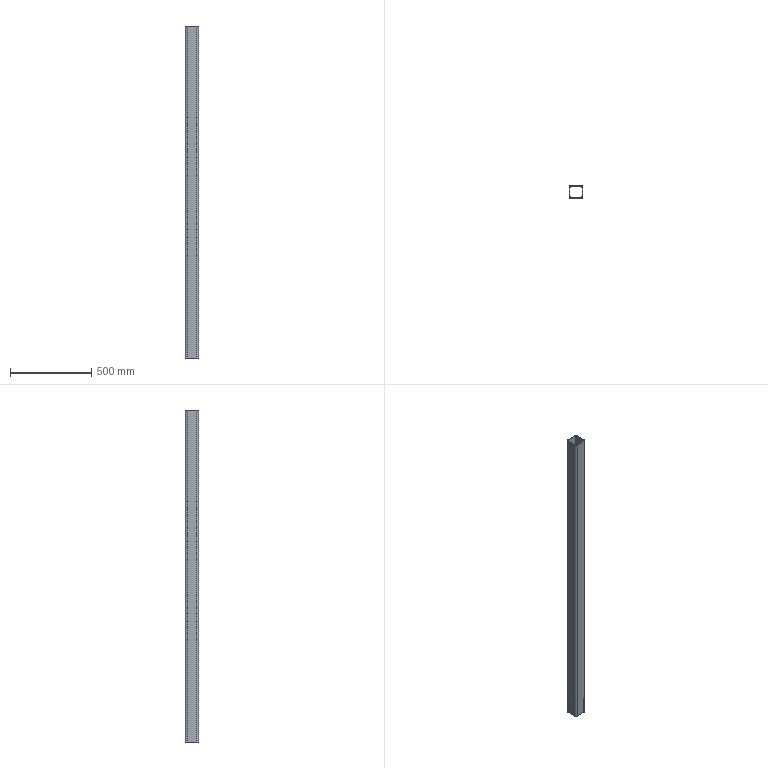Part | STEP file | 1 solid | 18 faces | box 80 x 80 x 2040 mm | volume 1795651 mm3 | plane 10 | cylinder 8 | commonest cylinder face diameters 14 x4 20 x4
STEP:
#1=CARTESIAN_POINT('',(0.,0.,0.));
#2=DIRECTION('',(0.,0.,1.));
#3=DIRECTION('',(1.,0.,0.));
#4=AXIS2_PLACEMENT_3D('',#1,#2,#3);
#5=CARTESIAN_POINT('',(-30.,40.,1020.));
#6=VERTEX_POINT('',#5);
#7=CARTESIAN_POINT('',(-40.,30.,1020.));
#8=VERTEX_POINT('',#7);
#9=CARTESIAN_POINT('',(-30.,30.,1020.));
#10=DIRECTION('',(0.,0.,1.));
#11=DIRECTION('',(1.,0.,0.));
#12=AXIS2_PLACEMENT_3D('',#9,#10,#11);
#13=CIRCLE('',#12,10.);
#14=CARTESIAN_POINT('',(-30.,30.,1020.));
#15=DIRECTION('',(0.,0.,1.));
#16=DIRECTION('',(1.,0.,0.));
#17=AXIS2_PLACEMENT_3D('',#14,#15,#16);
#18=PLANE('',#17);
#19=CARTESIAN_POINT('',(0.,0.));
#20=DIRECTION('',(1.,0.));
#21=AXIS2_PLACEMENT_2D('',#19,#20);
#22=CIRCLE('',#21,10.);
#23=(GEOMETRIC_REPRESENTATION_CONTEXT(2)PARAMETRIC_REPRESENTATION_CONTEXT()REPRESENTATION_CONTEXT('',''));
#24=DEFINITIONAL_REPRESENTATION('',(#22),#23);
#25=PCURVE('',#18,#24);
#26=CARTESIAN_POINT('',(-30.,30.,1020.));
#27=DIRECTION('',(0.,0.,-1.));
#28=DIRECTION('',(-1.,0.,0.));
#29=AXIS2_PLACEMENT_3D('',#26,#27,#28);
#30=CYLINDRICAL_SURFACE('',#29,10.);
#31=CARTESIAN_POINT('',(3.142,0.));
#32=DIRECTION('',(-1.,0.));
#33=VECTOR('',#32,1.);
#34=LINE('',#31,#33);
#35=(GEOMETRIC_REPRESENTATION_CONTEXT(2)PARAMETRIC_REPRESENTATION_CONTEXT()REPRESENTATION_CONTEXT('',''));
#36=DEFINITIONAL_REPRESENTATION('',(#34),#35);
#37=PCURVE('',#30,#36);
#38=SURFACE_CURVE('',#13,(#25,#37),.PCURVE_S1.);
#39=EDGE_CURVE('',#6,#8,#38,.T.);
#40=ORIENTED_EDGE('',*,*,#39,.T.);
#41=CARTESIAN_POINT('',(-40.,-30.,1020.));
#42=VERTEX_POINT('',#41);
#43=CARTESIAN_POINT('',(-40.,30.,1020.));
#44=DIRECTION('',(0.,-1.,0.));
#45=VECTOR('',#44,1.);
#46=LINE('',#43,#45);
#47=CARTESIAN_POINT('',(-10.,0.));
#48=DIRECTION('',(0.,-1.));
#49=VECTOR('',#48,1.);
#50=LINE('',#47,#49);
#51=(GEOMETRIC_REPRESENTATION_CONTEXT(2)PARAMETRIC_REPRESENTATION_CONTEXT()REPRESENTATION_CONTEXT('',''));
#52=DEFINITIONAL_REPRESENTATION('',(#50),#51);
#53=PCURVE('',#18,#52);
#54=CARTESIAN_POINT('',(-40.,30.,1020.));
#55=DIRECTION('',(1.,0.,0.));
#56=DIRECTION('',(0.,1.,0.));
#57=AXIS2_PLACEMENT_3D('',#54,#55,#56);
#58=PLANE('',#57);
#59=CARTESIAN_POINT('',(0.,0.));
#60=DIRECTION('',(-1.,0.));
#61=VECTOR('',#60,1.);
#62=LINE('',#59,#61);
#63=(GEOMETRIC_REPRESENTATION_CONTEXT(2)PARAMETRIC_REPRESENTATION_CONTEXT()REPRESENTATION_CONTEXT('',''));
#64=DEFINITIONAL_REPRESENTATION('',(#62),#63);
#65=PCURVE('',#58,#64);
#66=SURFACE_CURVE('',#46,(#53,#65),.PCURVE_S1.);
#67=EDGE_CURVE('',#8,#42,#66,.T.);
#68=ORIENTED_EDGE('',*,*,#67,.T.);
#69=CARTESIAN_POINT('',(-30.,-40.,1020.));
#70=VERTEX_POINT('',#69);
#71=CARTESIAN_POINT('',(-30.,-30.,1020.));
#72=DIRECTION('',(0.,0.,1.));
#73=DIRECTION('',(-1.,0.,0.));
#74=AXIS2_PLACEMENT_3D('',#71,#72,#73);
#75=CIRCLE('',#74,10.);
#76=CARTESIAN_POINT('',(0.,-60.));
#77=DIRECTION('',(-1.,0.));
#78=AXIS2_PLACEMENT_2D('',#76,#77);
#79=CIRCLE('',#78,10.);
#80=(GEOMETRIC_REPRESENTATION_CONTEXT(2)PARAMETRIC_REPRESENTATION_CONTEXT()REPRESENTATION_CONTEXT('',''));
#81=DEFINITIONAL_REPRESENTATION('',(#79),#80);
#82=PCURVE('',#18,#81);
#83=CARTESIAN_POINT('',(-30.,-30.,1020.));
#84=DIRECTION('',(0.,0.,-1.));
#85=DIRECTION('',(-1.,0.,0.));
#86=AXIS2_PLACEMENT_3D('',#83,#84,#85);
#87=CYLINDRICAL_SURFACE('',#86,10.);
#88=CARTESIAN_POINT('',(6.283,0.));
#89=DIRECTION('',(-1.,0.));
#90=VECTOR('',#89,1.);
#91=LINE('',#88,#90);
#92=(GEOMETRIC_REPRESENTATION_CONTEXT(2)PARAMETRIC_REPRESENTATION_CONTEXT()REPRESENTATION_CONTEXT('',''));
#93=DEFINITIONAL_REPRESENTATION('',(#91),#92);
#94=PCURVE('',#87,#93);
#95=SURFACE_CURVE('',#75,(#82,#94),.PCURVE_S1.);
#96=EDGE_CURVE('',#42,#70,#95,.T.);
#97=ORIENTED_EDGE('',*,*,#96,.T.);
#98=CARTESIAN_POINT('',(30.,-40.,1020.));
#99=VERTEX_POINT('',#98);
#100=CARTESIAN_POINT('',(30.,-40.,1020.));
#101=DIRECTION('',(1.,0.,0.));
#102=VECTOR('',#101,1.);
#103=LINE('',#100,#102);
#104=CARTESIAN_POINT('',(60.,-70.));
#105=DIRECTION('',(1.,0.));
#106=VECTOR('',#105,1.);
#107=LINE('',#104,#106);
#108=(GEOMETRIC_REPRESENTATION_CONTEXT(2)PARAMETRIC_REPRESENTATION_CONTEXT()REPRESENTATION_CONTEXT('',''));
#109=DEFINITIONAL_REPRESENTATION('',(#107),#108);
#110=PCURVE('',#18,#109);
#111=CARTESIAN_POINT('',(30.,-40.,1020.));
#112=DIRECTION('',(0.,1.,0.));
#113=DIRECTION('',(-1.,0.,0.));
#114=AXIS2_PLACEMENT_3D('',#111,#112,#113);
#115=PLANE('',#114);
#116=CARTESIAN_POINT('',(0.,0.));
#117=DIRECTION('',(-1.,0.));
#118=VECTOR('',#117,1.);
#119=LINE('',#116,#118);
#120=(GEOMETRIC_REPRESENTATION_CONTEXT(2)PARAMETRIC_REPRESENTATION_CONTEXT()REPRESENTATION_CONTEXT('',''));
#121=DEFINITIONAL_REPRESENTATION('',(#119),#120);
#122=PCURVE('',#115,#121);
#123=SURFACE_CURVE('',#103,(#110,#122),.PCURVE_S1.);
#124=EDGE_CURVE('',#70,#99,#123,.T.);
#125=ORIENTED_EDGE('',*,*,#124,.T.);
#126=CARTESIAN_POINT('',(40.,-30.,1020.));
#127=VERTEX_POINT('',#126);
#128=CARTESIAN_POINT('',(30.,-30.,1020.));
#129=DIRECTION('',(0.,0.,1.));
#130=DIRECTION('',(-1.,0.,0.));
#131=AXIS2_PLACEMENT_3D('',#128,#129,#130);
#132=CIRCLE('',#131,10.);
#133=CARTESIAN_POINT('',(60.,-60.));
#134=DIRECTION('',(-1.,0.));
#135=AXIS2_PLACEMENT_2D('',#133,#134);
#136=CIRCLE('',#135,10.);
#137=(GEOMETRIC_REPRESENTATION_CONTEXT(2)PARAMETRIC_REPRESENTATION_CONTEXT()REPRESENTATION_CONTEXT('',''));
#138=DEFINITIONAL_REPRESENTATION('',(#136),#137);
#139=PCURVE('',#18,#138);
#140=CARTESIAN_POINT('',(30.,-30.,1020.));
#141=DIRECTION('',(0.,0.,-1.));
#142=DIRECTION('',(-1.,0.,0.));
#143=AXIS2_PLACEMENT_3D('',#140,#141,#142);
#144=CYLINDRICAL_SURFACE('',#143,10.);
#145=CARTESIAN_POINT('',(6.283,0.));
#146=DIRECTION('',(-1.,0.));
#147=VECTOR('',#146,1.);
#148=LINE('',#145,#147);
#149=(GEOMETRIC_REPRESENTATION_CONTEXT(2)PARAMETRIC_REPRESENTATION_CONTEXT()REPRESENTATION_CONTEXT('',''));
#150=DEFINITIONAL_REPRESENTATION('',(#148),#149);
#151=PCURVE('',#144,#150);
#152=SURFACE_CURVE('',#132,(#139,#151),.PCURVE_S1.);
#153=EDGE_CURVE('',#99,#127,#152,.T.);
#154=ORIENTED_EDGE('',*,*,#153,.T.);
#155=CARTESIAN_POINT('',(40.,30.,1020.));
#156=VERTEX_POINT('',#155);
#157=CARTESIAN_POINT('',(40.,30.,1020.));
#158=DIRECTION('',(0.,1.,0.));
#159=VECTOR('',#158,1.);
#160=LINE('',#157,#159);
#161=CARTESIAN_POINT('',(70.,0.));
#162=DIRECTION('',(0.,1.));
#163=VECTOR('',#162,1.);
#164=LINE('',#161,#163);
#165=(GEOMETRIC_REPRESENTATION_CONTEXT(2)PARAMETRIC_REPRESENTATION_CONTEXT()REPRESENTATION_CONTEXT('',''));
#166=DEFINITIONAL_REPRESENTATION('',(#164),#165);
#167=PCURVE('',#18,#166);
#168=CARTESIAN_POINT('',(40.,30.,1020.));
#169=DIRECTION('',(-1.,0.,0.));
#170=DIRECTION('',(0.,-1.,0.));
#171=AXIS2_PLACEMENT_3D('',#168,#169,#170);
#172=PLANE('',#171);
#173=CARTESIAN_POINT('',(0.,0.));
#174=DIRECTION('',(-1.,0.));
#175=VECTOR('',#174,1.);
#176=LINE('',#173,#175);
#177=(GEOMETRIC_REPRESENTATION_CONTEXT(2)PARAMETRIC_REPRESENTATION_CONTEXT()REPRESENTATION_CONTEXT('',''));
#178=DEFINITIONAL_REPRESENTATION('',(#176),#177);
#179=PCURVE('',#172,#178);
#180=SURFACE_CURVE('',#160,(#167,#179),.PCURVE_S1.);
#181=EDGE_CURVE('',#127,#156,#180,.T.);
#182=ORIENTED_EDGE('',*,*,#181,.T.);
#183=CARTESIAN_POINT('',(30.,40.,1020.));
#184=VERTEX_POINT('',#183);
#185=CARTESIAN_POINT('',(30.,30.,1020.));
#186=DIRECTION('',(0.,0.,1.));
#187=DIRECTION('',(-1.,0.,0.));
#188=AXIS2_PLACEMENT_3D('',#185,#186,#187);
#189=CIRCLE('',#188,10.);
#190=CARTESIAN_POINT('',(60.,0.));
#191=DIRECTION('',(-1.,0.));
#192=AXIS2_PLACEMENT_2D('',#190,#191);
#193=CIRCLE('',#192,10.);
#194=(GEOMETRIC_REPRESENTATION_CONTEXT(2)PARAMETRIC_REPRESENTATION_CONTEXT()REPRESENTATION_CONTEXT('',''));
#195=DEFINITIONAL_REPRESENTATION('',(#193),#194);
#196=PCURVE('',#18,#195);
#197=CARTESIAN_POINT('',(30.,30.,1020.));
#198=DIRECTION('',(0.,0.,-1.));
#199=DIRECTION('',(-1.,0.,0.));
#200=AXIS2_PLACEMENT_3D('',#197,#198,#199);
#201=CYLINDRICAL_SURFACE('',#200,10.);
#202=CARTESIAN_POINT('',(6.283,0.));
#203=DIRECTION('',(-1.,0.));
#204=VECTOR('',#203,1.);
#205=LINE('',#202,#204);
#206=(GEOMETRIC_REPRESENTATION_CONTEXT(2)PARAMETRIC_REPRESENTATION_CONTEXT()REPRESENTATION_CONTEXT('',''));
#207=DEFINITIONAL_REPRESENTATION('',(#205),#206);
#208=PCURVE('',#201,#207);
#209=SURFACE_CURVE('',#189,(#196,#208),.PCURVE_S1.);
#210=EDGE_CURVE('',#156,#184,#209,.T.);
#211=ORIENTED_EDGE('',*,*,#210,.T.);
#212=CARTESIAN_POINT('',(30.,40.,1020.));
#213=DIRECTION('',(-1.,0.,0.));
#214=VECTOR('',#213,1.);
#215=LINE('',#212,#214);
#216=CARTESIAN_POINT('',(60.,10.));
#217=DIRECTION('',(-1.,0.));
#218=VECTOR('',#217,1.);
#219=LINE('',#216,#218);
#220=(GEOMETRIC_REPRESENTATION_CONTEXT(2)PARAMETRIC_REPRESENTATION_CONTEXT()REPRESENTATION_CONTEXT('',''));
#221=DEFINITIONAL_REPRESENTATION('',(#219),#220);
#222=PCURVE('',#18,#221);
#223=CARTESIAN_POINT('',(30.,40.,1020.));
#224=DIRECTION('',(0.,-1.,0.));
#225=DIRECTION('',(1.,0.,0.));
#226=AXIS2_PLACEMENT_3D('',#223,#224,#225);
#227=PLANE('',#226);
#228=CARTESIAN_POINT('',(0.,0.));
#229=DIRECTION('',(-1.,0.));
#230=VECTOR('',#229,1.);
#231=LINE('',#228,#230);
#232=(GEOMETRIC_REPRESENTATION_CONTEXT(2)PARAMETRIC_REPRESENTATION_CONTEXT()REPRESENTATION_CONTEXT('',''));
#233=DEFINITIONAL_REPRESENTATION('',(#231),#232);
#234=PCURVE('',#227,#233);
#235=SURFACE_CURVE('',#215,(#222,#234),.PCURVE_S1.);
#236=EDGE_CURVE('',#184,#6,#235,.T.);
#237=ORIENTED_EDGE('',*,*,#236,.T.);
#238=EDGE_LOOP('',(#40,#68,#97,#125,#154,#182,#211,#237));
#239=FACE_BOUND('',#238,.T.);
#240=CARTESIAN_POINT('',(30.,37.,1020.));
#241=VERTEX_POINT('',#240);
#242=CARTESIAN_POINT('',(-30.,37.,1020.));
#243=VERTEX_POINT('',#242);
#244=CARTESIAN_POINT('',(30.,37.,1020.));
#245=DIRECTION('',(-1.,0.,0.));
#246=VECTOR('',#245,1.);
#247=LINE('',#244,#246);
#248=CARTESIAN_POINT('',(60.,7.));
#249=DIRECTION('',(-1.,0.));
#250=VECTOR('',#249,1.);
#251=LINE('',#248,#250);
#252=(GEOMETRIC_REPRESENTATION_CONTEXT(2)PARAMETRIC_REPRESENTATION_CONTEXT()REPRESENTATION_CONTEXT('',''));
#253=DEFINITIONAL_REPRESENTATION('',(#251),#252);
#254=PCURVE('',#18,#253);
#255=CARTESIAN_POINT('',(30.,37.,1020.));
#256=DIRECTION('',(0.,-1.,0.));
#257=DIRECTION('',(0.,0.,-1.));
#258=AXIS2_PLACEMENT_3D('',#255,#256,#257);
#259=PLANE('',#258);
#260=CARTESIAN_POINT('',(0.,0.));
#261=DIRECTION('',(0.,-1.));
#262=VECTOR('',#261,1.);
#263=LINE('',#260,#262);
#264=(GEOMETRIC_REPRESENTATION_CONTEXT(2)PARAMETRIC_REPRESENTATION_CONTEXT()REPRESENTATION_CONTEXT('',''));
#265=DEFINITIONAL_REPRESENTATION('',(#263),#264);
#266=PCURVE('',#259,#265);
#267=SURFACE_CURVE('',#247,(#254,#266),.PCURVE_S1.);
#268=EDGE_CURVE('',#241,#243,#267,.T.);
#269=ORIENTED_EDGE('',*,*,#268,.F.);
#270=CARTESIAN_POINT('',(37.,30.,1020.));
#271=VERTEX_POINT('',#270);
#272=CARTESIAN_POINT('',(30.,30.,1020.));
#273=DIRECTION('',(0.,0.,1.));
#274=DIRECTION('',(-1.,0.,0.));
#275=AXIS2_PLACEMENT_3D('',#272,#273,#274);
#276=CIRCLE('',#275,7.);
#277=CARTESIAN_POINT('',(60.,0.));
#278=DIRECTION('',(-1.,0.));
#279=AXIS2_PLACEMENT_2D('',#277,#278);
#280=CIRCLE('',#279,7.);
#281=(GEOMETRIC_REPRESENTATION_CONTEXT(2)PARAMETRIC_REPRESENTATION_CONTEXT()REPRESENTATION_CONTEXT('',''));
#282=DEFINITIONAL_REPRESENTATION('',(#280),#281);
#283=PCURVE('',#18,#282);
#284=CARTESIAN_POINT('',(30.,30.,1020.));
#285=DIRECTION('',(0.,0.,-1.));
#286=DIRECTION('',(-1.,0.,0.));
#287=AXIS2_PLACEMENT_3D('',#284,#285,#286);
#288=CYLINDRICAL_SURFACE('',#287,7.);
#289=CARTESIAN_POINT('',(6.283,0.));
#290=DIRECTION('',(-1.,0.));
#291=VECTOR('',#290,1.);
#292=LINE('',#289,#291);
#293=(GEOMETRIC_REPRESENTATION_CONTEXT(2)PARAMETRIC_REPRESENTATION_CONTEXT()REPRESENTATION_CONTEXT('',''));
#294=DEFINITIONAL_REPRESENTATION('',(#292),#293);
#295=PCURVE('',#288,#294);
#296=SURFACE_CURVE('',#276,(#283,#295),.PCURVE_S1.);
#297=EDGE_CURVE('',#271,#241,#296,.T.);
#298=ORIENTED_EDGE('',*,*,#297,.F.);
#299=CARTESIAN_POINT('',(37.,-30.,1020.));
#300=VERTEX_POINT('',#299);
#301=CARTESIAN_POINT('',(37.,30.,1020.));
#302=DIRECTION('',(0.,1.,0.));
#303=VECTOR('',#302,1.);
#304=LINE('',#301,#303);
#305=CARTESIAN_POINT('',(67.,0.));
#306=DIRECTION('',(0.,1.));
#307=VECTOR('',#306,1.);
#308=LINE('',#305,#307);
#309=(GEOMETRIC_REPRESENTATION_CONTEXT(2)PARAMETRIC_REPRESENTATION_CONTEXT()REPRESENTATION_CONTEXT('',''));
#310=DEFINITIONAL_REPRESENTATION('',(#308),#309);
#311=PCURVE('',#18,#310);
#312=CARTESIAN_POINT('',(37.,30.,1020.));
#313=DIRECTION('',(-1.,0.,0.));
#314=DIRECTION('',(0.,-1.,0.));
#315=AXIS2_PLACEMENT_3D('',#312,#313,#314);
#316=PLANE('',#315);
#317=CARTESIAN_POINT('',(0.,0.));
#318=DIRECTION('',(-1.,0.));
#319=VECTOR('',#318,1.);
#320=LINE('',#317,#319);
#321=(GEOMETRIC_REPRESENTATION_CONTEXT(2)PARAMETRIC_REPRESENTATION_CONTEXT()REPRESENTATION_CONTEXT('',''));
#322=DEFINITIONAL_REPRESENTATION('',(#320),#321);
#323=PCURVE('',#316,#322);
#324=SURFACE_CURVE('',#304,(#311,#323),.PCURVE_S1.);
#325=EDGE_CURVE('',#300,#271,#324,.T.);
#326=ORIENTED_EDGE('',*,*,#325,.F.);
#327=CARTESIAN_POINT('',(30.,-37.,1020.));
#328=VERTEX_POINT('',#327);
#329=CARTESIAN_POINT('',(30.,-30.,1020.));
#330=DIRECTION('',(0.,0.,1.));
#331=DIRECTION('',(-1.,0.,0.));
#332=AXIS2_PLACEMENT_3D('',#329,#330,#331);
#333=CIRCLE('',#332,7.);
#334=CARTESIAN_POINT('',(60.,-60.));
#335=DIRECTION('',(-1.,0.));
#336=AXIS2_PLACEMENT_2D('',#334,#335);
#337=CIRCLE('',#336,7.);
#338=(GEOMETRIC_REPRESENTATION_CONTEXT(2)PARAMETRIC_REPRESENTATION_CONTEXT()REPRESENTATION_CONTEXT('',''));
#339=DEFINITIONAL_REPRESENTATION('',(#337),#338);
#340=PCURVE('',#18,#339);
#341=CARTESIAN_POINT('',(30.,-30.,1020.));
#342=DIRECTION('',(0.,0.,-1.));
#343=DIRECTION('',(-1.,0.,0.));
#344=AXIS2_PLACEMENT_3D('',#341,#342,#343);
#345=CYLINDRICAL_SURFACE('',#344,7.);
#346=CARTESIAN_POINT('',(6.283,0.));
#347=DIRECTION('',(-1.,0.));
#348=VECTOR('',#347,1.);
#349=LINE('',#346,#348);
#350=(GEOMETRIC_REPRESENTATION_CONTEXT(2)PARAMETRIC_REPRESENTATION_CONTEXT()REPRESENTATION_CONTEXT('',''));
#351=DEFINITIONAL_REPRESENTATION('',(#349),#350);
#352=PCURVE('',#345,#351);
#353=SURFACE_CURVE('',#333,(#340,#352),.PCURVE_S1.);
#354=EDGE_CURVE('',#328,#300,#353,.T.);
#355=ORIENTED_EDGE('',*,*,#354,.F.);
#356=CARTESIAN_POINT('',(-30.,-37.,1020.));
#357=VERTEX_POINT('',#356);
#358=CARTESIAN_POINT('',(30.,-37.,1020.));
#359=DIRECTION('',(1.,0.,0.));
#360=VECTOR('',#359,1.);
#361=LINE('',#358,#360);
#362=CARTESIAN_POINT('',(60.,-67.));
#363=DIRECTION('',(1.,0.));
#364=VECTOR('',#363,1.);
#365=LINE('',#362,#364);
#366=(GEOMETRIC_REPRESENTATION_CONTEXT(2)PARAMETRIC_REPRESENTATION_CONTEXT()REPRESENTATION_CONTEXT('',''));
#367=DEFINITIONAL_REPRESENTATION('',(#365),#366);
#368=PCURVE('',#18,#367);
#369=CARTESIAN_POINT('',(30.,-37.,1020.));
#370=DIRECTION('',(0.,1.,0.));
#371=DIRECTION('',(-1.,0.,0.));
#372=AXIS2_PLACEMENT_3D('',#369,#370,#371);
#373=PLANE('',#372);
#374=CARTESIAN_POINT('',(0.,0.));
#375=DIRECTION('',(-1.,0.));
#376=VECTOR('',#375,1.);
#377=LINE('',#374,#376);
#378=(GEOMETRIC_REPRESENTATION_CONTEXT(2)PARAMETRIC_REPRESENTATION_CONTEXT()REPRESENTATION_CONTEXT('',''));
#379=DEFINITIONAL_REPRESENTATION('',(#377),#378);
#380=PCURVE('',#373,#379);
#381=SURFACE_CURVE('',#361,(#368,#380),.PCURVE_S1.);
#382=EDGE_CURVE('',#357,#328,#381,.T.);
#383=ORIENTED_EDGE('',*,*,#382,.F.);
#384=CARTESIAN_POINT('',(-37.,-30.,1020.));
#385=VERTEX_POINT('',#384);
#386=CARTESIAN_POINT('',(-30.,-30.,1020.));
#387=DIRECTION('',(0.,0.,1.));
#388=DIRECTION('',(-1.,0.,0.));
#389=AXIS2_PLACEMENT_3D('',#386,#387,#388);
#390=CIRCLE('',#389,7.);
#391=CARTESIAN_POINT('',(0.,-60.));
#392=DIRECTION('',(-1.,0.));
#393=AXIS2_PLACEMENT_2D('',#391,#392);
#394=CIRCLE('',#393,7.);
#395=(GEOMETRIC_REPRESENTATION_CONTEXT(2)PARAMETRIC_REPRESENTATION_CONTEXT()REPRESENTATION_CONTEXT('',''));
#396=DEFINITIONAL_REPRESENTATION('',(#394),#395);
#397=PCURVE('',#18,#396);
#398=CARTESIAN_POINT('',(-30.,-30.,1020.));
#399=DIRECTION('',(0.,0.,-1.));
#400=DIRECTION('',(-1.,0.,0.));
#401=AXIS2_PLACEMENT_3D('',#398,#399,#400);
#402=CYLINDRICAL_SURFACE('',#401,7.);
#403=CARTESIAN_POINT('',(6.283,0.));
#404=DIRECTION('',(-1.,0.));
#405=VECTOR('',#404,1.);
#406=LINE('',#403,#405);
#407=(GEOMETRIC_REPRESENTATION_CONTEXT(2)PARAMETRIC_REPRESENTATION_CONTEXT()REPRESENTATION_CONTEXT('',''));
#408=DEFINITIONAL_REPRESENTATION('',(#406),#407);
#409=PCURVE('',#402,#408);
#410=SURFACE_CURVE('',#390,(#397,#409),.PCURVE_S1.);
#411=EDGE_CURVE('',#385,#357,#410,.T.);
#412=ORIENTED_EDGE('',*,*,#411,.F.);
#413=CARTESIAN_POINT('',(-37.,30.,1020.));
#414=VERTEX_POINT('',#413);
#415=CARTESIAN_POINT('',(-37.,30.,1020.));
#416=DIRECTION('',(0.,-1.,0.));
#417=VECTOR('',#416,1.);
#418=LINE('',#415,#417);
#419=CARTESIAN_POINT('',(-7.,0.));
#420=DIRECTION('',(0.,-1.));
#421=VECTOR('',#420,1.);
#422=LINE('',#419,#421);
#423=(GEOMETRIC_REPRESENTATION_CONTEXT(2)PARAMETRIC_REPRESENTATION_CONTEXT()REPRESENTATION_CONTEXT('',''));
#424=DEFINITIONAL_REPRESENTATION('',(#422),#423);
#425=PCURVE('',#18,#424);
#426=CARTESIAN_POINT('',(-37.,30.,1020.));
#427=DIRECTION('',(1.,0.,0.));
#428=DIRECTION('',(0.,0.,-1.));
#429=AXIS2_PLACEMENT_3D('',#426,#427,#428);
#430=PLANE('',#429);
#431=CARTESIAN_POINT('',(0.,0.));
#432=DIRECTION('',(0.,-1.));
#433=VECTOR('',#432,1.);
#434=LINE('',#431,#433);
#435=(GEOMETRIC_REPRESENTATION_CONTEXT(2)PARAMETRIC_REPRESENTATION_CONTEXT()REPRESENTATION_CONTEXT('',''));
#436=DEFINITIONAL_REPRESENTATION('',(#434),#435);
#437=PCURVE('',#430,#436);
#438=SURFACE_CURVE('',#418,(#425,#437),.PCURVE_S1.);
#439=EDGE_CURVE('',#414,#385,#438,.T.);
#440=ORIENTED_EDGE('',*,*,#439,.F.);
#441=CARTESIAN_POINT('',(-30.,30.,1020.));
#442=DIRECTION('',(0.,0.,1.));
#443=DIRECTION('',(1.,0.,0.));
#444=AXIS2_PLACEMENT_3D('',#441,#442,#443);
#445=CIRCLE('',#444,7.);
#446=CARTESIAN_POINT('',(0.,0.));
#447=DIRECTION('',(1.,0.));
#448=AXIS2_PLACEMENT_2D('',#446,#447);
#449=CIRCLE('',#448,7.);
#450=(GEOMETRIC_REPRESENTATION_CONTEXT(2)PARAMETRIC_REPRESENTATION_CONTEXT()REPRESENTATION_CONTEXT('',''));
#451=DEFINITIONAL_REPRESENTATION('',(#449),#450);
#452=PCURVE('',#18,#451);
#453=CARTESIAN_POINT('',(-30.,30.,1020.));
#454=DIRECTION('',(0.,0.,-1.));
#455=DIRECTION('',(-1.,0.,0.));
#456=AXIS2_PLACEMENT_3D('',#453,#454,#455);
#457=CYLINDRICAL_SURFACE('',#456,7.);
#458=CARTESIAN_POINT('',(3.142,0.));
#459=DIRECTION('',(-1.,0.));
#460=VECTOR('',#459,1.);
#461=LINE('',#458,#460);
#462=(GEOMETRIC_REPRESENTATION_CONTEXT(2)PARAMETRIC_REPRESENTATION_CONTEXT()REPRESENTATION_CONTEXT('',''));
#463=DEFINITIONAL_REPRESENTATION('',(#461),#462);
#464=PCURVE('',#457,#463);
#465=SURFACE_CURVE('',#445,(#452,#464),.PCURVE_S1.);
#466=EDGE_CURVE('',#243,#414,#465,.T.);
#467=ORIENTED_EDGE('',*,*,#466,.F.);
#468=EDGE_LOOP('',(#269,#298,#326,#355,#383,#412,#440,#467));
#469=FACE_BOUND('',#468,.T.);
#470=ADVANCED_FACE('',(#239,#469),#18,.T.);
#471=CARTESIAN_POINT('',(-30.,40.,-1020.));
#472=VERTEX_POINT('',#471);
#473=CARTESIAN_POINT('',(-40.,30.,-1020.));
#474=VERTEX_POINT('',#473);
#475=CARTESIAN_POINT('',(-30.,30.,-1020.));
#476=DIRECTION('',(0.,0.,1.));
#477=DIRECTION('',(1.,0.,0.));
#478=AXIS2_PLACEMENT_3D('',#475,#476,#477);
#479=CIRCLE('',#478,10.);
#480=CARTESIAN_POINT('',(-30.,30.,-1020.));
#481=DIRECTION('',(0.,0.,1.));
#482=DIRECTION('',(1.,0.,0.));
#483=AXIS2_PLACEMENT_3D('',#480,#481,#482);
#484=PLANE('',#483);
#485=CARTESIAN_POINT('',(0.,0.));
#486=DIRECTION('',(1.,0.));
#487=AXIS2_PLACEMENT_2D('',#485,#486);
#488=CIRCLE('',#487,10.);
#489=(GEOMETRIC_REPRESENTATION_CONTEXT(2)PARAMETRIC_REPRESENTATION_CONTEXT()REPRESENTATION_CONTEXT('',''));
#490=DEFINITIONAL_REPRESENTATION('',(#488),#489);
#491=PCURVE('',#484,#490);
#492=CARTESIAN_POINT('',(3.142,2040.));
#493=DIRECTION('',(-1.,0.));
#494=VECTOR('',#493,1.);
#495=LINE('',#492,#494);
#496=(GEOMETRIC_REPRESENTATION_CONTEXT(2)PARAMETRIC_REPRESENTATION_CONTEXT()REPRESENTATION_CONTEXT('',''));
#497=DEFINITIONAL_REPRESENTATION('',(#495),#496);
#498=PCURVE('',#30,#497);
#499=SURFACE_CURVE('',#479,(#491,#498),.PCURVE_S1.);
#500=EDGE_CURVE('',#472,#474,#499,.T.);
#501=ORIENTED_EDGE('',*,*,#500,.F.);
#502=CARTESIAN_POINT('',(30.,40.,-1020.));
#503=VERTEX_POINT('',#502);
#504=CARTESIAN_POINT('',(30.,40.,-1020.));
#505=DIRECTION('',(-1.,0.,0.));
#506=VECTOR('',#505,1.);
#507=LINE('',#504,#506);
#508=CARTESIAN_POINT('',(60.,10.));
#509=DIRECTION('',(-1.,0.));
#510=VECTOR('',#509,1.);
#511=LINE('',#508,#510);
#512=(GEOMETRIC_REPRESENTATION_CONTEXT(2)PARAMETRIC_REPRESENTATION_CONTEXT()REPRESENTATION_CONTEXT('',''));
#513=DEFINITIONAL_REPRESENTATION('',(#511),#512);
#514=PCURVE('',#484,#513);
#515=CARTESIAN_POINT('',(0.,-2040.));
#516=DIRECTION('',(-1.,0.));
#517=VECTOR('',#516,1.);
#518=LINE('',#515,#517);
#519=(GEOMETRIC_REPRESENTATION_CONTEXT(2)PARAMETRIC_REPRESENTATION_CONTEXT()REPRESENTATION_CONTEXT('',''));
#520=DEFINITIONAL_REPRESENTATION('',(#518),#519);
#521=PCURVE('',#227,#520);
#522=SURFACE_CURVE('',#507,(#514,#521),.PCURVE_S1.);
#523=EDGE_CURVE('',#503,#472,#522,.T.);
#524=ORIENTED_EDGE('',*,*,#523,.F.);
#525=CARTESIAN_POINT('',(40.,30.,-1020.));
#526=VERTEX_POINT('',#525);
#527=CARTESIAN_POINT('',(30.,30.,-1020.));
#528=DIRECTION('',(0.,0.,1.));
#529=DIRECTION('',(-1.,0.,0.));
#530=AXIS2_PLACEMENT_3D('',#527,#528,#529);
#531=CIRCLE('',#530,10.);
#532=CARTESIAN_POINT('',(60.,0.));
#533=DIRECTION('',(-1.,0.));
#534=AXIS2_PLACEMENT_2D('',#532,#533);
#535=CIRCLE('',#534,10.);
#536=(GEOMETRIC_REPRESENTATION_CONTEXT(2)PARAMETRIC_REPRESENTATION_CONTEXT()REPRESENTATION_CONTEXT('',''));
#537=DEFINITIONAL_REPRESENTATION('',(#535),#536);
#538=PCURVE('',#484,#537);
#539=CARTESIAN_POINT('',(6.283,2040.));
#540=DIRECTION('',(-1.,0.));
#541=VECTOR('',#540,1.);
#542=LINE('',#539,#541);
#543=(GEOMETRIC_REPRESENTATION_CONTEXT(2)PARAMETRIC_REPRESENTATION_CONTEXT()REPRESENTATION_CONTEXT('',''));
#544=DEFINITIONAL_REPRESENTATION('',(#542),#543);
#545=PCURVE('',#201,#544);
#546=SURFACE_CURVE('',#531,(#538,#545),.PCURVE_S1.);
#547=EDGE_CURVE('',#526,#503,#546,.T.);
#548=ORIENTED_EDGE('',*,*,#547,.F.);
#549=CARTESIAN_POINT('',(40.,-30.,-1020.));
#550=VERTEX_POINT('',#549);
#551=CARTESIAN_POINT('',(40.,30.,-1020.));
#552=DIRECTION('',(0.,1.,0.));
#553=VECTOR('',#552,1.);
#554=LINE('',#551,#553);
#555=CARTESIAN_POINT('',(70.,0.));
#556=DIRECTION('',(0.,1.));
#557=VECTOR('',#556,1.);
#558=LINE('',#555,#557);
#559=(GEOMETRIC_REPRESENTATION_CONTEXT(2)PARAMETRIC_REPRESENTATION_CONTEXT()REPRESENTATION_CONTEXT('',''));
#560=DEFINITIONAL_REPRESENTATION('',(#558),#559);
#561=PCURVE('',#484,#560);
#562=CARTESIAN_POINT('',(0.,-2040.));
#563=DIRECTION('',(-1.,0.));
#564=VECTOR('',#563,1.);
#565=LINE('',#562,#564);
#566=(GEOMETRIC_REPRESENTATION_CONTEXT(2)PARAMETRIC_REPRESENTATION_CONTEXT()REPRESENTATION_CONTEXT('',''));
#567=DEFINITIONAL_REPRESENTATION('',(#565),#566);
#568=PCURVE('',#172,#567);
#569=SURFACE_CURVE('',#554,(#561,#568),.PCURVE_S1.);
#570=EDGE_CURVE('',#550,#526,#569,.T.);
#571=ORIENTED_EDGE('',*,*,#570,.F.);
#572=CARTESIAN_POINT('',(30.,-40.,-1020.));
#573=VERTEX_POINT('',#572);
#574=CARTESIAN_POINT('',(30.,-30.,-1020.));
#575=DIRECTION('',(0.,0.,1.));
#576=DIRECTION('',(-1.,0.,0.));
#577=AXIS2_PLACEMENT_3D('',#574,#575,#576);
#578=CIRCLE('',#577,10.);
#579=CARTESIAN_POINT('',(60.,-60.));
#580=DIRECTION('',(-1.,0.));
#581=AXIS2_PLACEMENT_2D('',#579,#580);
#582=CIRCLE('',#581,10.);
#583=(GEOMETRIC_REPRESENTATION_CONTEXT(2)PARAMETRIC_REPRESENTATION_CONTEXT()REPRESENTATION_CONTEXT('',''));
#584=DEFINITIONAL_REPRESENTATION('',(#582),#583);
#585=PCURVE('',#484,#584);
#586=CARTESIAN_POINT('',(6.283,2040.));
#587=DIRECTION('',(-1.,0.));
#588=VECTOR('',#587,1.);
#589=LINE('',#586,#588);
#590=(GEOMETRIC_REPRESENTATION_CONTEXT(2)PARAMETRIC_REPRESENTATION_CONTEXT()REPRESENTATION_CONTEXT('',''));
#591=DEFINITIONAL_REPRESENTATION('',(#589),#590);
#592=PCURVE('',#144,#591);
#593=SURFACE_CURVE('',#578,(#585,#592),.PCURVE_S1.);
#594=EDGE_CURVE('',#573,#550,#593,.T.);
#595=ORIENTED_EDGE('',*,*,#594,.F.);
#596=CARTESIAN_POINT('',(-30.,-40.,-1020.));
#597=VERTEX_POINT('',#596);
#598=CARTESIAN_POINT('',(30.,-40.,-1020.));
#599=DIRECTION('',(1.,0.,0.));
#600=VECTOR('',#599,1.);
#601=LINE('',#598,#600);
#602=CARTESIAN_POINT('',(60.,-70.));
#603=DIRECTION('',(1.,0.));
#604=VECTOR('',#603,1.);
#605=LINE('',#602,#604);
#606=(GEOMETRIC_REPRESENTATION_CONTEXT(2)PARAMETRIC_REPRESENTATION_CONTEXT()REPRESENTATION_CONTEXT('',''));
#607=DEFINITIONAL_REPRESENTATION('',(#605),#606);
#608=PCURVE('',#484,#607);
#609=CARTESIAN_POINT('',(0.,-2040.));
#610=DIRECTION('',(-1.,0.));
#611=VECTOR('',#610,1.);
#612=LINE('',#609,#611);
#613=(GEOMETRIC_REPRESENTATION_CONTEXT(2)PARAMETRIC_REPRESENTATION_CONTEXT()REPRESENTATION_CONTEXT('',''));
#614=DEFINITIONAL_REPRESENTATION('',(#612),#613);
#615=PCURVE('',#115,#614);
#616=SURFACE_CURVE('',#601,(#608,#615),.PCURVE_S1.);
#617=EDGE_CURVE('',#597,#573,#616,.T.);
#618=ORIENTED_EDGE('',*,*,#617,.F.);
#619=CARTESIAN_POINT('',(-40.,-30.,-1020.));
#620=VERTEX_POINT('',#619);
#621=CARTESIAN_POINT('',(-30.,-30.,-1020.));
#622=DIRECTION('',(0.,0.,1.));
#623=DIRECTION('',(-1.,0.,0.));
#624=AXIS2_PLACEMENT_3D('',#621,#622,#623);
#625=CIRCLE('',#624,10.);
#626=CARTESIAN_POINT('',(0.,-60.));
#627=DIRECTION('',(-1.,0.));
#628=AXIS2_PLACEMENT_2D('',#626,#627);
#629=CIRCLE('',#628,10.);
#630=(GEOMETRIC_REPRESENTATION_CONTEXT(2)PARAMETRIC_REPRESENTATION_CONTEXT()REPRESENTATION_CONTEXT('',''));
#631=DEFINITIONAL_REPRESENTATION('',(#629),#630);
#632=PCURVE('',#484,#631);
#633=CARTESIAN_POINT('',(6.283,2040.));
#634=DIRECTION('',(-1.,0.));
#635=VECTOR('',#634,1.);
#636=LINE('',#633,#635);
#637=(GEOMETRIC_REPRESENTATION_CONTEXT(2)PARAMETRIC_REPRESENTATION_CONTEXT()REPRESENTATION_CONTEXT('',''));
#638=DEFINITIONAL_REPRESENTATION('',(#636),#637);
#639=PCURVE('',#87,#638);
#640=SURFACE_CURVE('',#625,(#632,#639),.PCURVE_S1.);
#641=EDGE_CURVE('',#620,#597,#640,.T.);
#642=ORIENTED_EDGE('',*,*,#641,.F.);
#643=CARTESIAN_POINT('',(-40.,30.,-1020.));
#644=DIRECTION('',(0.,-1.,0.));
#645=VECTOR('',#644,1.);
#646=LINE('',#643,#645);
#647=CARTESIAN_POINT('',(-10.,0.));
#648=DIRECTION('',(0.,-1.));
#649=VECTOR('',#648,1.);
#650=LINE('',#647,#649);
#651=(GEOMETRIC_REPRESENTATION_CONTEXT(2)PARAMETRIC_REPRESENTATION_CONTEXT()REPRESENTATION_CONTEXT('',''));
#652=DEFINITIONAL_REPRESENTATION('',(#650),#651);
#653=PCURVE('',#484,#652);
#654=CARTESIAN_POINT('',(0.,-2040.));
#655=DIRECTION('',(-1.,0.));
#656=VECTOR('',#655,1.);
#657=LINE('',#654,#656);
#658=(GEOMETRIC_REPRESENTATION_CONTEXT(2)PARAMETRIC_REPRESENTATION_CONTEXT()REPRESENTATION_CONTEXT('',''));
#659=DEFINITIONAL_REPRESENTATION('',(#657),#658);
#660=PCURVE('',#58,#659);
#661=SURFACE_CURVE('',#646,(#653,#660),.PCURVE_S1.);
#662=EDGE_CURVE('',#474,#620,#661,.T.);
#663=ORIENTED_EDGE('',*,*,#662,.F.);
#664=EDGE_LOOP('',(#501,#524,#548,#571,#595,#618,#642,#663));
#665=FACE_BOUND('',#664,.T.);
#666=CARTESIAN_POINT('',(37.,30.,-1020.));
#667=VERTEX_POINT('',#666);
#668=CARTESIAN_POINT('',(30.,37.,-1020.));
#669=VERTEX_POINT('',#668);
#670=CARTESIAN_POINT('',(30.,30.,-1020.));
#671=DIRECTION('',(0.,0.,1.));
#672=DIRECTION('',(-1.,0.,0.));
#673=AXIS2_PLACEMENT_3D('',#670,#671,#672);
#674=CIRCLE('',#673,7.);
#675=CARTESIAN_POINT('',(60.,0.));
#676=DIRECTION('',(-1.,0.));
#677=AXIS2_PLACEMENT_2D('',#675,#676);
#678=CIRCLE('',#677,7.);
#679=(GEOMETRIC_REPRESENTATION_CONTEXT(2)PARAMETRIC_REPRESENTATION_CONTEXT()REPRESENTATION_CONTEXT('',''));
#680=DEFINITIONAL_REPRESENTATION('',(#678),#679);
#681=PCURVE('',#484,#680);
#682=CARTESIAN_POINT('',(6.283,2040.));
#683=DIRECTION('',(-1.,0.));
#684=VECTOR('',#683,1.);
#685=LINE('',#682,#684);
#686=(GEOMETRIC_REPRESENTATION_CONTEXT(2)PARAMETRIC_REPRESENTATION_CONTEXT()REPRESENTATION_CONTEXT('',''));
#687=DEFINITIONAL_REPRESENTATION('',(#685),#686);
#688=PCURVE('',#288,#687);
#689=SURFACE_CURVE('',#674,(#681,#688),.PCURVE_S1.);
#690=EDGE_CURVE('',#667,#669,#689,.T.);
#691=ORIENTED_EDGE('',*,*,#690,.T.);
#692=CARTESIAN_POINT('',(-30.,37.,-1020.));
#693=VERTEX_POINT('',#692);
#694=CARTESIAN_POINT('',(30.,37.,-1020.));
#695=DIRECTION('',(-1.,0.,0.));
#696=VECTOR('',#695,1.);
#697=LINE('',#694,#696);
#698=CARTESIAN_POINT('',(60.,7.));
#699=DIRECTION('',(-1.,0.));
#700=VECTOR('',#699,1.);
#701=LINE('',#698,#700);
#702=(GEOMETRIC_REPRESENTATION_CONTEXT(2)PARAMETRIC_REPRESENTATION_CONTEXT()REPRESENTATION_CONTEXT('',''));
#703=DEFINITIONAL_REPRESENTATION('',(#701),#702);
#704=PCURVE('',#484,#703);
#705=CARTESIAN_POINT('',(2040.,0.));
#706=DIRECTION('',(0.,-1.));
#707=VECTOR('',#706,1.);
#708=LINE('',#705,#707);
#709=(GEOMETRIC_REPRESENTATION_CONTEXT(2)PARAMETRIC_REPRESENTATION_CONTEXT()REPRESENTATION_CONTEXT('',''));
#710=DEFINITIONAL_REPRESENTATION('',(#708),#709);
#711=PCURVE('',#259,#710);
#712=SURFACE_CURVE('',#697,(#704,#711),.PCURVE_S1.);
#713=EDGE_CURVE('',#669,#693,#712,.T.);
#714=ORIENTED_EDGE('',*,*,#713,.T.);
#715=CARTESIAN_POINT('',(-37.,30.,-1020.));
#716=VERTEX_POINT('',#715);
#717=CARTESIAN_POINT('',(-30.,30.,-1020.));
#718=DIRECTION('',(0.,0.,1.));
#719=DIRECTION('',(1.,0.,0.));
#720=AXIS2_PLACEMENT_3D('',#717,#718,#719);
#721=CIRCLE('',#720,7.);
#722=CARTESIAN_POINT('',(0.,0.));
#723=DIRECTION('',(1.,0.));
#724=AXIS2_PLACEMENT_2D('',#722,#723);
#725=CIRCLE('',#724,7.);
#726=(GEOMETRIC_REPRESENTATION_CONTEXT(2)PARAMETRIC_REPRESENTATION_CONTEXT()REPRESENTATION_CONTEXT('',''));
#727=DEFINITIONAL_REPRESENTATION('',(#725),#726);
#728=PCURVE('',#484,#727);
#729=CARTESIAN_POINT('',(3.142,2040.));
#730=DIRECTION('',(-1.,0.));
#731=VECTOR('',#730,1.);
#732=LINE('',#729,#731);
#733=(GEOMETRIC_REPRESENTATION_CONTEXT(2)PARAMETRIC_REPRESENTATION_CONTEXT()REPRESENTATION_CONTEXT('',''));
#734=DEFINITIONAL_REPRESENTATION('',(#732),#733);
#735=PCURVE('',#457,#734);
#736=SURFACE_CURVE('',#721,(#728,#735),.PCURVE_S1.);
#737=EDGE_CURVE('',#693,#716,#736,.T.);
#738=ORIENTED_EDGE('',*,*,#737,.T.);
#739=CARTESIAN_POINT('',(-37.,-30.,-1020.));
#740=VERTEX_POINT('',#739);
#741=CARTESIAN_POINT('',(-37.,30.,-1020.));
#742=DIRECTION('',(0.,-1.,0.));
#743=VECTOR('',#742,1.);
#744=LINE('',#741,#743);
#745=CARTESIAN_POINT('',(-7.,0.));
#746=DIRECTION('',(0.,-1.));
#747=VECTOR('',#746,1.);
#748=LINE('',#745,#747);
#749=(GEOMETRIC_REPRESENTATION_CONTEXT(2)PARAMETRIC_REPRESENTATION_CONTEXT()REPRESENTATION_CONTEXT('',''));
#750=DEFINITIONAL_REPRESENTATION('',(#748),#749);
#751=PCURVE('',#484,#750);
#752=CARTESIAN_POINT('',(2040.,0.));
#753=DIRECTION('',(0.,-1.));
#754=VECTOR('',#753,1.);
#755=LINE('',#752,#754);
#756=(GEOMETRIC_REPRESENTATION_CONTEXT(2)PARAMETRIC_REPRESENTATION_CONTEXT()REPRESENTATION_CONTEXT('',''));
#757=DEFINITIONAL_REPRESENTATION('',(#755),#756);
#758=PCURVE('',#430,#757);
#759=SURFACE_CURVE('',#744,(#751,#758),.PCURVE_S1.);
#760=EDGE_CURVE('',#716,#740,#759,.T.);
#761=ORIENTED_EDGE('',*,*,#760,.T.);
#762=CARTESIAN_POINT('',(-30.,-37.,-1020.));
#763=VERTEX_POINT('',#762);
#764=CARTESIAN_POINT('',(-30.,-30.,-1020.));
#765=DIRECTION('',(0.,0.,1.));
#766=DIRECTION('',(-1.,0.,0.));
#767=AXIS2_PLACEMENT_3D('',#764,#765,#766);
#768=CIRCLE('',#767,7.);
#769=CARTESIAN_POINT('',(0.,-60.));
#770=DIRECTION('',(-1.,0.));
#771=AXIS2_PLACEMENT_2D('',#769,#770);
#772=CIRCLE('',#771,7.);
#773=(GEOMETRIC_REPRESENTATION_CONTEXT(2)PARAMETRIC_REPRESENTATION_CONTEXT()REPRESENTATION_CONTEXT('',''));
#774=DEFINITIONAL_REPRESENTATION('',(#772),#773);
#775=PCURVE('',#484,#774);
#776=CARTESIAN_POINT('',(6.283,2040.));
#777=DIRECTION('',(-1.,0.));
#778=VECTOR('',#777,1.);
#779=LINE('',#776,#778);
#780=(GEOMETRIC_REPRESENTATION_CONTEXT(2)PARAMETRIC_REPRESENTATION_CONTEXT()REPRESENTATION_CONTEXT('',''));
#781=DEFINITIONAL_REPRESENTATION('',(#779),#780);
#782=PCURVE('',#402,#781);
#783=SURFACE_CURVE('',#768,(#775,#782),.PCURVE_S1.);
#784=EDGE_CURVE('',#740,#763,#783,.T.);
#785=ORIENTED_EDGE('',*,*,#784,.T.);
#786=CARTESIAN_POINT('',(30.,-37.,-1020.));
#787=VERTEX_POINT('',#786);
#788=CARTESIAN_POINT('',(30.,-37.,-1020.));
#789=DIRECTION('',(1.,0.,0.));
#790=VECTOR('',#789,1.);
#791=LINE('',#788,#790);
#792=CARTESIAN_POINT('',(60.,-67.));
#793=DIRECTION('',(1.,0.));
#794=VECTOR('',#793,1.);
#795=LINE('',#792,#794);
#796=(GEOMETRIC_REPRESENTATION_CONTEXT(2)PARAMETRIC_REPRESENTATION_CONTEXT()REPRESENTATION_CONTEXT('',''));
#797=DEFINITIONAL_REPRESENTATION('',(#795),#796);
#798=PCURVE('',#484,#797);
#799=CARTESIAN_POINT('',(0.,-2040.));
#800=DIRECTION('',(-1.,0.));
#801=VECTOR('',#800,1.);
#802=LINE('',#799,#801);
#803=(GEOMETRIC_REPRESENTATION_CONTEXT(2)PARAMETRIC_REPRESENTATION_CONTEXT()REPRESENTATION_CONTEXT('',''));
#804=DEFINITIONAL_REPRESENTATION('',(#802),#803);
#805=PCURVE('',#373,#804);
#806=SURFACE_CURVE('',#791,(#798,#805),.PCURVE_S1.);
#807=EDGE_CURVE('',#763,#787,#806,.T.);
#808=ORIENTED_EDGE('',*,*,#807,.T.);
#809=CARTESIAN_POINT('',(37.,-30.,-1020.));
#810=VERTEX_POINT('',#809);
#811=CARTESIAN_POINT('',(30.,-30.,-1020.));
#812=DIRECTION('',(0.,0.,1.));
#813=DIRECTION('',(-1.,0.,0.));
#814=AXIS2_PLACEMENT_3D('',#811,#812,#813);
#815=CIRCLE('',#814,7.);
#816=CARTESIAN_POINT('',(60.,-60.));
#817=DIRECTION('',(-1.,0.));
#818=AXIS2_PLACEMENT_2D('',#816,#817);
#819=CIRCLE('',#818,7.);
#820=(GEOMETRIC_REPRESENTATION_CONTEXT(2)PARAMETRIC_REPRESENTATION_CONTEXT()REPRESENTATION_CONTEXT('',''));
#821=DEFINITIONAL_REPRESENTATION('',(#819),#820);
#822=PCURVE('',#484,#821);
#823=CARTESIAN_POINT('',(6.283,2040.));
#824=DIRECTION('',(-1.,0.));
#825=VECTOR('',#824,1.);
#826=LINE('',#823,#825);
#827=(GEOMETRIC_REPRESENTATION_CONTEXT(2)PARAMETRIC_REPRESENTATION_CONTEXT()REPRESENTATION_CONTEXT('',''));
#828=DEFINITIONAL_REPRESENTATION('',(#826),#827);
#829=PCURVE('',#345,#828);
#830=SURFACE_CURVE('',#815,(#822,#829),.PCURVE_S1.);
#831=EDGE_CURVE('',#787,#810,#830,.T.);
#832=ORIENTED_EDGE('',*,*,#831,.T.);
#833=CARTESIAN_POINT('',(37.,30.,-1020.));
#834=DIRECTION('',(0.,1.,0.));
#835=VECTOR('',#834,1.);
#836=LINE('',#833,#835);
#837=CARTESIAN_POINT('',(67.,0.));
#838=DIRECTION('',(0.,1.));
#839=VECTOR('',#838,1.);
#840=LINE('',#837,#839);
#841=(GEOMETRIC_REPRESENTATION_CONTEXT(2)PARAMETRIC_REPRESENTATION_CONTEXT()REPRESENTATION_CONTEXT('',''));
#842=DEFINITIONAL_REPRESENTATION('',(#840),#841);
#843=PCURVE('',#484,#842);
#844=CARTESIAN_POINT('',(0.,-2040.));
#845=DIRECTION('',(-1.,0.));
#846=VECTOR('',#845,1.);
#847=LINE('',#844,#846);
#848=(GEOMETRIC_REPRESENTATION_CONTEXT(2)PARAMETRIC_REPRESENTATION_CONTEXT()REPRESENTATION_CONTEXT('',''));
#849=DEFINITIONAL_REPRESENTATION('',(#847),#848);
#850=PCURVE('',#316,#849);
#851=SURFACE_CURVE('',#836,(#843,#850),.PCURVE_S1.);
#852=EDGE_CURVE('',#810,#667,#851,.T.);
#853=ORIENTED_EDGE('',*,*,#852,.T.);
#854=EDGE_LOOP('',(#691,#714,#738,#761,#785,#808,#832,#853));
#855=FACE_BOUND('',#854,.T.);
#856=ADVANCED_FACE('',(#665,#855),#484,.F.);
#857=ORIENTED_EDGE('',*,*,#500,.T.);
#858=CARTESIAN_POINT('',(-40.,30.,1020.));
#859=DIRECTION('',(0.,0.,-1.));
#860=VECTOR('',#859,1.);
#861=LINE('',#858,#860);
#862=CARTESIAN_POINT('',(0.,0.));
#863=DIRECTION('',(0.,1.));
#864=VECTOR('',#863,1.);
#865=LINE('',#862,#864);
#866=(GEOMETRIC_REPRESENTATION_CONTEXT(2)PARAMETRIC_REPRESENTATION_CONTEXT()REPRESENTATION_CONTEXT('',''));
#867=DEFINITIONAL_REPRESENTATION('',(#865),#866);
#868=PCURVE('',#30,#867);
#869=CARTESIAN_POINT('',(0.,0.));
#870=DIRECTION('',(0.,-1.));
#871=VECTOR('',#870,1.);
#872=LINE('',#869,#871);
#873=(GEOMETRIC_REPRESENTATION_CONTEXT(2)PARAMETRIC_REPRESENTATION_CONTEXT()REPRESENTATION_CONTEXT('',''));
#874=DEFINITIONAL_REPRESENTATION('',(#872),#873);
#875=PCURVE('',#58,#874);
#876=SURFACE_CURVE('',#861,(#868,#875),.PCURVE_S1.);
#877=EDGE_CURVE('',#8,#474,#876,.T.);
#878=ORIENTED_EDGE('',*,*,#877,.F.);
#879=ORIENTED_EDGE('',*,*,#39,.F.);
#880=CARTESIAN_POINT('',(-30.,40.,1020.));
#881=DIRECTION('',(0.,0.,-1.));
#882=VECTOR('',#881,1.);
#883=LINE('',#880,#882);
#884=CARTESIAN_POINT('',(1.571,0.));
#885=DIRECTION('',(0.,1.));
#886=VECTOR('',#885,1.);
#887=LINE('',#884,#886);
#888=(GEOMETRIC_REPRESENTATION_CONTEXT(2)PARAMETRIC_REPRESENTATION_CONTEXT()REPRESENTATION_CONTEXT('',''));
#889=DEFINITIONAL_REPRESENTATION('',(#887),#888);
#890=PCURVE('',#30,#889);
#891=CARTESIAN_POINT('',(-60.,0.));
#892=DIRECTION('',(0.,-1.));
#893=VECTOR('',#892,1.);
#894=LINE('',#891,#893);
#895=(GEOMETRIC_REPRESENTATION_CONTEXT(2)PARAMETRIC_REPRESENTATION_CONTEXT()REPRESENTATION_CONTEXT('',''));
#896=DEFINITIONAL_REPRESENTATION('',(#894),#895);
#897=PCURVE('',#227,#896);
#898=SURFACE_CURVE('',#883,(#890,#897),.PCURVE_S1.);
#899=EDGE_CURVE('',#6,#472,#898,.T.);
#900=ORIENTED_EDGE('',*,*,#899,.T.);
#901=EDGE_LOOP('',(#857,#878,#879,#900));
#902=FACE_BOUND('',#901,.T.);
#903=ADVANCED_FACE('',(#902),#30,.T.);
#904=ORIENTED_EDGE('',*,*,#662,.T.);
#905=CARTESIAN_POINT('',(-40.,-30.,1020.));
#906=DIRECTION('',(0.,0.,-1.));
#907=VECTOR('',#906,1.);
#908=LINE('',#905,#907);
#909=CARTESIAN_POINT('',(-60.,0.));
#910=DIRECTION('',(0.,-1.));
#911=VECTOR('',#910,1.);
#912=LINE('',#909,#911);
#913=(GEOMETRIC_REPRESENTATION_CONTEXT(2)PARAMETRIC_REPRESENTATION_CONTEXT()REPRESENTATION_CONTEXT('',''));
#914=DEFINITIONAL_REPRESENTATION('',(#912),#913);
#915=PCURVE('',#58,#914);
#916=CARTESIAN_POINT('',(6.283,0.));
#917=DIRECTION('',(0.,1.));
#918=VECTOR('',#917,1.);
#919=LINE('',#916,#918);
#920=(GEOMETRIC_REPRESENTATION_CONTEXT(2)PARAMETRIC_REPRESENTATION_CONTEXT()REPRESENTATION_CONTEXT('',''));
#921=DEFINITIONAL_REPRESENTATION('',(#919),#920);
#922=PCURVE('',#87,#921);
#923=SURFACE_CURVE('',#908,(#915,#922),.PCURVE_S1.);
#924=EDGE_CURVE('',#42,#620,#923,.T.);
#925=ORIENTED_EDGE('',*,*,#924,.F.);
#926=ORIENTED_EDGE('',*,*,#67,.F.);
#927=ORIENTED_EDGE('',*,*,#877,.T.);
#928=EDGE_LOOP('',(#904,#925,#926,#927));
#929=FACE_BOUND('',#928,.T.);
#930=ADVANCED_FACE('',(#929),#58,.F.);
#931=ORIENTED_EDGE('',*,*,#641,.T.);
#932=CARTESIAN_POINT('',(-30.,-40.,1020.));
#933=DIRECTION('',(0.,0.,-1.));
#934=VECTOR('',#933,1.);
#935=LINE('',#932,#934);
#936=CARTESIAN_POINT('',(4.712,0.));
#937=DIRECTION('',(0.,1.));
#938=VECTOR('',#937,1.);
#939=LINE('',#936,#938);
#940=(GEOMETRIC_REPRESENTATION_CONTEXT(2)PARAMETRIC_REPRESENTATION_CONTEXT()REPRESENTATION_CONTEXT('',''));
#941=DEFINITIONAL_REPRESENTATION('',(#939),#940);
#942=PCURVE('',#87,#941);
#943=CARTESIAN_POINT('',(60.,0.));
#944=DIRECTION('',(0.,-1.));
#945=VECTOR('',#944,1.);
#946=LINE('',#943,#945);
#947=(GEOMETRIC_REPRESENTATION_CONTEXT(2)PARAMETRIC_REPRESENTATION_CONTEXT()REPRESENTATION_CONTEXT('',''));
#948=DEFINITIONAL_REPRESENTATION('',(#946),#947);
#949=PCURVE('',#115,#948);
#950=SURFACE_CURVE('',#935,(#942,#949),.PCURVE_S1.);
#951=EDGE_CURVE('',#70,#597,#950,.T.);
#952=ORIENTED_EDGE('',*,*,#951,.F.);
#953=ORIENTED_EDGE('',*,*,#96,.F.);
#954=ORIENTED_EDGE('',*,*,#924,.T.);
#955=EDGE_LOOP('',(#931,#952,#953,#954));
#956=FACE_BOUND('',#955,.T.);
#957=ADVANCED_FACE('',(#956),#87,.T.);
#958=ORIENTED_EDGE('',*,*,#617,.T.);
#959=CARTESIAN_POINT('',(30.,-40.,1020.));
#960=DIRECTION('',(0.,0.,-1.));
#961=VECTOR('',#960,1.);
#962=LINE('',#959,#961);
#963=CARTESIAN_POINT('',(0.,0.));
#964=DIRECTION('',(0.,-1.));
#965=VECTOR('',#964,1.);
#966=LINE('',#963,#965);
#967=(GEOMETRIC_REPRESENTATION_CONTEXT(2)PARAMETRIC_REPRESENTATION_CONTEXT()REPRESENTATION_CONTEXT('',''));
#968=DEFINITIONAL_REPRESENTATION('',(#966),#967);
#969=PCURVE('',#115,#968);
#970=CARTESIAN_POINT('',(4.712,0.));
#971=DIRECTION('',(0.,1.));
#972=VECTOR('',#971,1.);
#973=LINE('',#970,#972);
#974=(GEOMETRIC_REPRESENTATION_CONTEXT(2)PARAMETRIC_REPRESENTATION_CONTEXT()REPRESENTATION_CONTEXT('',''));
#975=DEFINITIONAL_REPRESENTATION('',(#973),#974);
#976=PCURVE('',#144,#975);
#977=SURFACE_CURVE('',#962,(#969,#976),.PCURVE_S1.);
#978=EDGE_CURVE('',#99,#573,#977,.T.);
#979=ORIENTED_EDGE('',*,*,#978,.F.);
#980=ORIENTED_EDGE('',*,*,#124,.F.);
#981=ORIENTED_EDGE('',*,*,#951,.T.);
#982=EDGE_LOOP('',(#958,#979,#980,#981));
#983=FACE_BOUND('',#982,.T.);
#984=ADVANCED_FACE('',(#983),#115,.F.);
#985=ORIENTED_EDGE('',*,*,#594,.T.);
#986=CARTESIAN_POINT('',(40.,-30.,1020.));
#987=DIRECTION('',(0.,0.,-1.));
#988=VECTOR('',#987,1.);
#989=LINE('',#986,#988);
#990=CARTESIAN_POINT('',(3.142,0.));
#991=DIRECTION('',(0.,1.));
#992=VECTOR('',#991,1.);
#993=LINE('',#990,#992);
#994=(GEOMETRIC_REPRESENTATION_CONTEXT(2)PARAMETRIC_REPRESENTATION_CONTEXT()REPRESENTATION_CONTEXT('',''));
#995=DEFINITIONAL_REPRESENTATION('',(#993),#994);
#996=PCURVE('',#144,#995);
#997=CARTESIAN_POINT('',(60.,0.));
#998=DIRECTION('',(0.,-1.));
#999=VECTOR('',#998,1.);
#1000=LINE('',#997,#999);
#1001=(GEOMETRIC_REPRESENTATION_CONTEXT(2)PARAMETRIC_REPRESENTATION_CONTEXT()REPRESENTATION_CONTEXT('',''));
#1002=DEFINITIONAL_REPRESENTATION('',(#1000),#1001);
#1003=PCURVE('',#172,#1002);
#1004=SURFACE_CURVE('',#989,(#996,#1003),.PCURVE_S1.);
#1005=EDGE_CURVE('',#127,#550,#1004,.T.);
#1006=ORIENTED_EDGE('',*,*,#1005,.F.);
#1007=ORIENTED_EDGE('',*,*,#153,.F.);
#1008=ORIENTED_EDGE('',*,*,#978,.T.);
#1009=EDGE_LOOP('',(#985,#1006,#1007,#1008));
#1010=FACE_BOUND('',#1009,.T.);
#1011=ADVANCED_FACE('',(#1010),#144,.T.);
#1012=ORIENTED_EDGE('',*,*,#570,.T.);
#1013=CARTESIAN_POINT('',(40.,30.,1020.));
#1014=DIRECTION('',(0.,0.,-1.));
#1015=VECTOR('',#1014,1.);
#1016=LINE('',#1013,#1015);
#1017=CARTESIAN_POINT('',(0.,0.));
#1018=DIRECTION('',(0.,-1.));
#1019=VECTOR('',#1018,1.);
#1020=LINE('',#1017,#1019);
#1021=(GEOMETRIC_REPRESENTATION_CONTEXT(2)PARAMETRIC_REPRESENTATION_CONTEXT()REPRESENTATION_CONTEXT('',''));
#1022=DEFINITIONAL_REPRESENTATION('',(#1020),#1021);
#1023=PCURVE('',#172,#1022);
#1024=CARTESIAN_POINT('',(3.142,0.));
#1025=DIRECTION('',(0.,1.));
#1026=VECTOR('',#1025,1.);
#1027=LINE('',#1024,#1026);
#1028=(GEOMETRIC_REPRESENTATION_CONTEXT(2)PARAMETRIC_REPRESENTATION_CONTEXT()REPRESENTATION_CONTEXT('',''));
#1029=DEFINITIONAL_REPRESENTATION('',(#1027),#1028);
#1030=PCURVE('',#201,#1029);
#1031=SURFACE_CURVE('',#1016,(#1023,#1030),.PCURVE_S1.);
#1032=EDGE_CURVE('',#156,#526,#1031,.T.);
#1033=ORIENTED_EDGE('',*,*,#1032,.F.);
#1034=ORIENTED_EDGE('',*,*,#181,.F.);
#1035=ORIENTED_EDGE('',*,*,#1005,.T.);
#1036=EDGE_LOOP('',(#1012,#1033,#1034,#1035));
#1037=FACE_BOUND('',#1036,.T.);
#1038=ADVANCED_FACE('',(#1037),#172,.F.);
#1039=ORIENTED_EDGE('',*,*,#547,.T.);
#1040=CARTESIAN_POINT('',(30.,40.,1020.));
#1041=DIRECTION('',(0.,0.,-1.));
#1042=VECTOR('',#1041,1.);
#1043=LINE('',#1040,#1042);
#1044=CARTESIAN_POINT('',(1.571,0.));
#1045=DIRECTION('',(0.,1.));
#1046=VECTOR('',#1045,1.);
#1047=LINE('',#1044,#1046);
#1048=(GEOMETRIC_REPRESENTATION_CONTEXT(2)PARAMETRIC_REPRESENTATION_CONTEXT()REPRESENTATION_CONTEXT('',''));
#1049=DEFINITIONAL_REPRESENTATION('',(#1047),#1048);
#1050=PCURVE('',#201,#1049);
#1051=CARTESIAN_POINT('',(0.,0.));
#1052=DIRECTION('',(0.,-1.));
#1053=VECTOR('',#1052,1.);
#1054=LINE('',#1051,#1053);
#1055=(GEOMETRIC_REPRESENTATION_CONTEXT(2)PARAMETRIC_REPRESENTATION_CONTEXT()REPRESENTATION_CONTEXT('',''));
#1056=DEFINITIONAL_REPRESENTATION('',(#1054),#1055);
#1057=PCURVE('',#227,#1056);
#1058=SURFACE_CURVE('',#1043,(#1050,#1057),.PCURVE_S1.);
#1059=EDGE_CURVE('',#184,#503,#1058,.T.);
#1060=ORIENTED_EDGE('',*,*,#1059,.F.);
#1061=ORIENTED_EDGE('',*,*,#210,.F.);
#1062=ORIENTED_EDGE('',*,*,#1032,.T.);
#1063=EDGE_LOOP('',(#1039,#1060,#1061,#1062));
#1064=FACE_BOUND('',#1063,.T.);
#1065=ADVANCED_FACE('',(#1064),#201,.T.);
#1066=ORIENTED_EDGE('',*,*,#523,.T.);
#1067=ORIENTED_EDGE('',*,*,#899,.F.);
#1068=ORIENTED_EDGE('',*,*,#236,.F.);
#1069=ORIENTED_EDGE('',*,*,#1059,.T.);
#1070=EDGE_LOOP('',(#1066,#1067,#1068,#1069));
#1071=FACE_BOUND('',#1070,.T.);
#1072=ADVANCED_FACE('',(#1071),#227,.F.);
#1073=CARTESIAN_POINT('',(30.,37.,1020.));
#1074=DIRECTION('',(0.,0.,-1.));
#1075=VECTOR('',#1074,1.);
#1076=LINE('',#1073,#1075);
#1077=CARTESIAN_POINT('',(1.571,0.));
#1078=DIRECTION('',(0.,1.));
#1079=VECTOR('',#1078,1.);
#1080=LINE('',#1077,#1079);
#1081=(GEOMETRIC_REPRESENTATION_CONTEXT(2)PARAMETRIC_REPRESENTATION_CONTEXT()REPRESENTATION_CONTEXT('',''));
#1082=DEFINITIONAL_REPRESENTATION('',(#1080),#1081);
#1083=PCURVE('',#288,#1082);
#1084=CARTESIAN_POINT('',(0.,0.));
#1085=DIRECTION('',(1.,0.));
#1086=VECTOR('',#1085,1.);
#1087=LINE('',#1084,#1086);
#1088=(GEOMETRIC_REPRESENTATION_CONTEXT(2)PARAMETRIC_REPRESENTATION_CONTEXT()REPRESENTATION_CONTEXT('',''));
#1089=DEFINITIONAL_REPRESENTATION('',(#1087),#1088);
#1090=PCURVE('',#259,#1089);
#1091=SURFACE_CURVE('',#1076,(#1083,#1090),.PCURVE_S1.);
#1092=EDGE_CURVE('',#241,#669,#1091,.T.);
#1093=ORIENTED_EDGE('',*,*,#1092,.F.);
#1094=ORIENTED_EDGE('',*,*,#297,.F.);
#1095=CARTESIAN_POINT('',(37.,30.,1020.));
#1096=DIRECTION('',(0.,0.,-1.));
#1097=VECTOR('',#1096,1.);
#1098=LINE('',#1095,#1097);
#1099=CARTESIAN_POINT('',(3.142,0.));
#1100=DIRECTION('',(0.,1.));
#1101=VECTOR('',#1100,1.);
#1102=LINE('',#1099,#1101);
#1103=(GEOMETRIC_REPRESENTATION_CONTEXT(2)PARAMETRIC_REPRESENTATION_CONTEXT()REPRESENTATION_CONTEXT('',''));
#1104=DEFINITIONAL_REPRESENTATION('',(#1102),#1103);
#1105=PCURVE('',#288,#1104);
#1106=CARTESIAN_POINT('',(0.,0.));
#1107=DIRECTION('',(0.,-1.));
#1108=VECTOR('',#1107,1.);
#1109=LINE('',#1106,#1108);
#1110=(GEOMETRIC_REPRESENTATION_CONTEXT(2)PARAMETRIC_REPRESENTATION_CONTEXT()REPRESENTATION_CONTEXT('',''));
#1111=DEFINITIONAL_REPRESENTATION('',(#1109),#1110);
#1112=PCURVE('',#316,#1111);
#1113=SURFACE_CURVE('',#1098,(#1105,#1112),.PCURVE_S1.);
#1114=EDGE_CURVE('',#271,#667,#1113,.T.);
#1115=ORIENTED_EDGE('',*,*,#1114,.T.);
#1116=ORIENTED_EDGE('',*,*,#690,.T.);
#1117=EDGE_LOOP('',(#1093,#1094,#1115,#1116));
#1118=FACE_BOUND('',#1117,.F.);
#1119=ADVANCED_FACE('',(#1118),#288,.F.);
#1120=ORIENTED_EDGE('',*,*,#713,.F.);
#1121=ORIENTED_EDGE('',*,*,#1092,.F.);
#1122=ORIENTED_EDGE('',*,*,#268,.T.);
#1123=CARTESIAN_POINT('',(-30.,37.,1020.));
#1124=DIRECTION('',(0.,0.,-1.));
#1125=VECTOR('',#1124,1.);
#1126=LINE('',#1123,#1125);
#1127=CARTESIAN_POINT('',(0.,-60.));
#1128=DIRECTION('',(1.,0.));
#1129=VECTOR('',#1128,1.);
#1130=LINE('',#1127,#1129);
#1131=(GEOMETRIC_REPRESENTATION_CONTEXT(2)PARAMETRIC_REPRESENTATION_CONTEXT()REPRESENTATION_CONTEXT('',''));
#1132=DEFINITIONAL_REPRESENTATION('',(#1130),#1131);
#1133=PCURVE('',#259,#1132);
#1134=CARTESIAN_POINT('',(1.571,0.));
#1135=DIRECTION('',(0.,1.));
#1136=VECTOR('',#1135,1.);
#1137=LINE('',#1134,#1136);
#1138=(GEOMETRIC_REPRESENTATION_CONTEXT(2)PARAMETRIC_REPRESENTATION_CONTEXT()REPRESENTATION_CONTEXT('',''));
#1139=DEFINITIONAL_REPRESENTATION('',(#1137),#1138);
#1140=PCURVE('',#457,#1139);
#1141=SURFACE_CURVE('',#1126,(#1133,#1140),.PCURVE_S1.);
#1142=EDGE_CURVE('',#243,#693,#1141,.T.);
#1143=ORIENTED_EDGE('',*,*,#1142,.T.);
#1144=EDGE_LOOP('',(#1120,#1121,#1122,#1143));
#1145=FACE_BOUND('',#1144,.T.);
#1146=ADVANCED_FACE('',(#1145),#259,.T.);
#1147=CARTESIAN_POINT('',(-37.,30.,1020.));
#1148=DIRECTION('',(0.,0.,-1.));
#1149=VECTOR('',#1148,1.);
#1150=LINE('',#1147,#1149);
#1151=CARTESIAN_POINT('',(0.,0.));
#1152=DIRECTION('',(0.,1.));
#1153=VECTOR('',#1152,1.);
#1154=LINE('',#1151,#1153);
#1155=(GEOMETRIC_REPRESENTATION_CONTEXT(2)PARAMETRIC_REPRESENTATION_CONTEXT()REPRESENTATION_CONTEXT('',''));
#1156=DEFINITIONAL_REPRESENTATION('',(#1154),#1155);
#1157=PCURVE('',#457,#1156);
#1158=CARTESIAN_POINT('',(0.,0.));
#1159=DIRECTION('',(1.,0.));
#1160=VECTOR('',#1159,1.);
#1161=LINE('',#1158,#1160);
#1162=(GEOMETRIC_REPRESENTATION_CONTEXT(2)PARAMETRIC_REPRESENTATION_CONTEXT()REPRESENTATION_CONTEXT('',''));
#1163=DEFINITIONAL_REPRESENTATION('',(#1161),#1162);
#1164=PCURVE('',#430,#1163);
#1165=SURFACE_CURVE('',#1150,(#1157,#1164),.PCURVE_S1.);
#1166=EDGE_CURVE('',#414,#716,#1165,.T.);
#1167=ORIENTED_EDGE('',*,*,#1166,.F.);
#1168=ORIENTED_EDGE('',*,*,#466,.F.);
#1169=ORIENTED_EDGE('',*,*,#1142,.T.);
#1170=ORIENTED_EDGE('',*,*,#737,.T.);
#1171=EDGE_LOOP('',(#1167,#1168,#1169,#1170));
#1172=FACE_BOUND('',#1171,.F.);
#1173=ADVANCED_FACE('',(#1172),#457,.F.);
#1174=ORIENTED_EDGE('',*,*,#760,.F.);
#1175=ORIENTED_EDGE('',*,*,#1166,.F.);
#1176=ORIENTED_EDGE('',*,*,#439,.T.);
#1177=CARTESIAN_POINT('',(-37.,-30.,1020.));
#1178=DIRECTION('',(0.,0.,-1.));
#1179=VECTOR('',#1178,1.);
#1180=LINE('',#1177,#1179);
#1181=CARTESIAN_POINT('',(0.,-60.));
#1182=DIRECTION('',(1.,0.));
#1183=VECTOR('',#1182,1.);
#1184=LINE('',#1181,#1183);
#1185=(GEOMETRIC_REPRESENTATION_CONTEXT(2)PARAMETRIC_REPRESENTATION_CONTEXT()REPRESENTATION_CONTEXT('',''));
#1186=DEFINITIONAL_REPRESENTATION('',(#1184),#1185);
#1187=PCURVE('',#430,#1186);
#1188=CARTESIAN_POINT('',(6.283,0.));
#1189=DIRECTION('',(0.,1.));
#1190=VECTOR('',#1189,1.);
#1191=LINE('',#1188,#1190);
#1192=(GEOMETRIC_REPRESENTATION_CONTEXT(2)PARAMETRIC_REPRESENTATION_CONTEXT()REPRESENTATION_CONTEXT('',''));
#1193=DEFINITIONAL_REPRESENTATION('',(#1191),#1192);
#1194=PCURVE('',#402,#1193);
#1195=SURFACE_CURVE('',#1180,(#1187,#1194),.PCURVE_S1.);
#1196=EDGE_CURVE('',#385,#740,#1195,.T.);
#1197=ORIENTED_EDGE('',*,*,#1196,.T.);
#1198=EDGE_LOOP('',(#1174,#1175,#1176,#1197));
#1199=FACE_BOUND('',#1198,.T.);
#1200=ADVANCED_FACE('',(#1199),#430,.T.);
#1201=CARTESIAN_POINT('',(-30.,-37.,1020.));
#1202=DIRECTION('',(0.,0.,-1.));
#1203=VECTOR('',#1202,1.);
#1204=LINE('',#1201,#1203);
#1205=CARTESIAN_POINT('',(4.712,0.));
#1206=DIRECTION('',(0.,1.));
#1207=VECTOR('',#1206,1.);
#1208=LINE('',#1205,#1207);
#1209=(GEOMETRIC_REPRESENTATION_CONTEXT(2)PARAMETRIC_REPRESENTATION_CONTEXT()REPRESENTATION_CONTEXT('',''));
#1210=DEFINITIONAL_REPRESENTATION('',(#1208),#1209);
#1211=PCURVE('',#402,#1210);
#1212=CARTESIAN_POINT('',(60.,0.));
#1213=DIRECTION('',(0.,-1.));
#1214=VECTOR('',#1213,1.);
#1215=LINE('',#1212,#1214);
#1216=(GEOMETRIC_REPRESENTATION_CONTEXT(2)PARAMETRIC_REPRESENTATION_CONTEXT()REPRESENTATION_CONTEXT('',''));
#1217=DEFINITIONAL_REPRESENTATION('',(#1215),#1216);
#1218=PCURVE('',#373,#1217);
#1219=SURFACE_CURVE('',#1204,(#1211,#1218),.PCURVE_S1.);
#1220=EDGE_CURVE('',#357,#763,#1219,.T.);
#1221=ORIENTED_EDGE('',*,*,#1220,.F.);
#1222=ORIENTED_EDGE('',*,*,#411,.F.);
#1223=ORIENTED_EDGE('',*,*,#1196,.T.);
#1224=ORIENTED_EDGE('',*,*,#784,.T.);
#1225=EDGE_LOOP('',(#1221,#1222,#1223,#1224));
#1226=FACE_BOUND('',#1225,.F.);
#1227=ADVANCED_FACE('',(#1226),#402,.F.);
#1228=ORIENTED_EDGE('',*,*,#807,.F.);
#1229=ORIENTED_EDGE('',*,*,#1220,.F.);
#1230=ORIENTED_EDGE('',*,*,#382,.T.);
#1231=CARTESIAN_POINT('',(30.,-37.,1020.));
#1232=DIRECTION('',(0.,0.,-1.));
#1233=VECTOR('',#1232,1.);
#1234=LINE('',#1231,#1233);
#1235=CARTESIAN_POINT('',(0.,0.));
#1236=DIRECTION('',(0.,-1.));
#1237=VECTOR('',#1236,1.);
#1238=LINE('',#1235,#1237);
#1239=(GEOMETRIC_REPRESENTATION_CONTEXT(2)PARAMETRIC_REPRESENTATION_CONTEXT()REPRESENTATION_CONTEXT('',''));
#1240=DEFINITIONAL_REPRESENTATION('',(#1238),#1239);
#1241=PCURVE('',#373,#1240);
#1242=CARTESIAN_POINT('',(4.712,0.));
#1243=DIRECTION('',(0.,1.));
#1244=VECTOR('',#1243,1.);
#1245=LINE('',#1242,#1244);
#1246=(GEOMETRIC_REPRESENTATION_CONTEXT(2)PARAMETRIC_REPRESENTATION_CONTEXT()REPRESENTATION_CONTEXT('',''));
#1247=DEFINITIONAL_REPRESENTATION('',(#1245),#1246);
#1248=PCURVE('',#345,#1247);
#1249=SURFACE_CURVE('',#1234,(#1241,#1248),.PCURVE_S1.);
#1250=EDGE_CURVE('',#328,#787,#1249,.T.);
#1251=ORIENTED_EDGE('',*,*,#1250,.T.);
#1252=EDGE_LOOP('',(#1228,#1229,#1230,#1251));
#1253=FACE_BOUND('',#1252,.T.);
#1254=ADVANCED_FACE('',(#1253),#373,.T.);
#1255=CARTESIAN_POINT('',(37.,-30.,1020.));
#1256=DIRECTION('',(0.,0.,-1.));
#1257=VECTOR('',#1256,1.);
#1258=LINE('',#1255,#1257);
#1259=CARTESIAN_POINT('',(3.142,0.));
#1260=DIRECTION('',(0.,1.));
#1261=VECTOR('',#1260,1.);
#1262=LINE('',#1259,#1261);
#1263=(GEOMETRIC_REPRESENTATION_CONTEXT(2)PARAMETRIC_REPRESENTATION_CONTEXT()REPRESENTATION_CONTEXT('',''));
#1264=DEFINITIONAL_REPRESENTATION('',(#1262),#1263);
#1265=PCURVE('',#345,#1264);
#1266=CARTESIAN_POINT('',(60.,0.));
#1267=DIRECTION('',(0.,-1.));
#1268=VECTOR('',#1267,1.);
#1269=LINE('',#1266,#1268);
#1270=(GEOMETRIC_REPRESENTATION_CONTEXT(2)PARAMETRIC_REPRESENTATION_CONTEXT()REPRESENTATION_CONTEXT('',''));
#1271=DEFINITIONAL_REPRESENTATION('',(#1269),#1270);
#1272=PCURVE('',#316,#1271);
#1273=SURFACE_CURVE('',#1258,(#1265,#1272),.PCURVE_S1.);
#1274=EDGE_CURVE('',#300,#810,#1273,.T.);
#1275=ORIENTED_EDGE('',*,*,#1274,.F.);
#1276=ORIENTED_EDGE('',*,*,#354,.F.);
#1277=ORIENTED_EDGE('',*,*,#1250,.T.);
#1278=ORIENTED_EDGE('',*,*,#831,.T.);
#1279=EDGE_LOOP('',(#1275,#1276,#1277,#1278));
#1280=FACE_BOUND('',#1279,.F.);
#1281=ADVANCED_FACE('',(#1280),#345,.F.);
#1282=ORIENTED_EDGE('',*,*,#852,.F.);
#1283=ORIENTED_EDGE('',*,*,#1274,.F.);
#1284=ORIENTED_EDGE('',*,*,#325,.T.);
#1285=ORIENTED_EDGE('',*,*,#1114,.T.);
#1286=EDGE_LOOP('',(#1282,#1283,#1284,#1285));
#1287=FACE_BOUND('',#1286,.T.);
#1288=ADVANCED_FACE('',(#1287),#316,.T.);
#1289=CLOSED_SHELL('',(#470,#856,#903,#930,#957,#984,#1011,#1038,#1065,#1072,#1119,#1146,#1173,#1200,#1227,#1254,#1281,#1288));
#1290=MANIFOLD_SOLID_BREP('',#1289);
#1291=(LENGTH_UNIT()NAMED_UNIT(*)SI_UNIT(.MILLI.,.METRE.));
#1292=UNCERTAINTY_MEASURE_WITH_UNIT(LENGTH_MEASURE(0.0000001),#1291,'','');
#1293=(NAMED_UNIT(*)PLANE_ANGLE_UNIT()SI_UNIT($,.RADIAN.));
#1294=(NAMED_UNIT(*)SI_UNIT($,.STERADIAN.)SOLID_ANGLE_UNIT());
#1295=(GEOMETRIC_REPRESENTATION_CONTEXT(3)GLOBAL_UNCERTAINTY_ASSIGNED_CONTEXT((#1292))GLOBAL_UNIT_ASSIGNED_CONTEXT((#1291,#1293,#1294))REPRESENTATION_CONTEXT('',''));
#1296=ADVANCED_BREP_SHAPE_REPRESENTATION('',(#4,#1290),#1295);